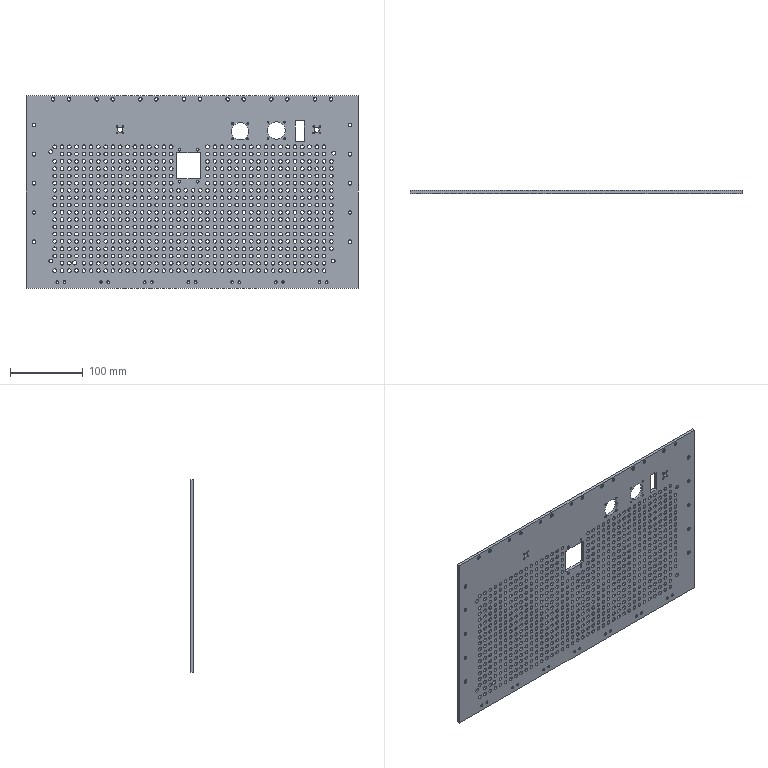Part | STEP file | Main chassis rear panel | 1 solid | 875 faces | box 456 x 4 x 264.7 mm | volume 416377 mm3 | cylinder 745 | cone 116 | plane 14 | commonest cylinder face diameters 5 x670 4.3 x24 3.2 x18 1.6 x8 2.05 x8 2 x4